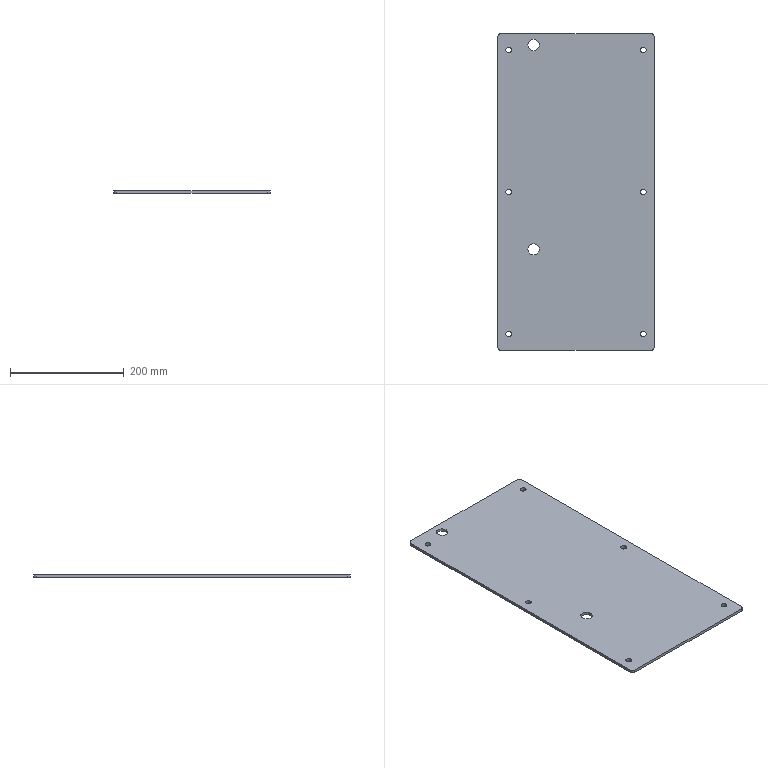Part | SolidWorks | features BaseBody 1 | 1 solid | 26 faces | box 275 x 558 x 5 mm | volume 761645 mm3 | cylinder 20 | plane 6 | commonest cylinder face diameters 10 x16 20 x4
STEP:
#1=CARTESIAN_POINT('',(-64.75,-101.,5.));
#2=VERTEX_POINT('',#1);
#3=CARTESIAN_POINT('',(-84.75,-101.,5.));
#4=VERTEX_POINT('',#3);
#5=CARTESIAN_POINT('',(-74.75,-101.,5.));
#6=DIRECTION('',(0.,0.,-1.));
#7=DIRECTION('',(-1.,0.,0.));
#8=AXIS2_PLACEMENT_3D('',#5,#6,#7);
#9=CIRCLE('',#8,10.);
#10=EDGE_CURVE('',#2,#4,#9,.T.);
#11=ORIENTED_EDGE('',*,*,#10,.F.);
#12=CARTESIAN_POINT('',(-64.75,-101.,0.));
#13=VERTEX_POINT('',#12);
#14=CARTESIAN_POINT('',(-64.75,-101.,10.));
#15=DIRECTION('',(0.,0.,-1.));
#16=VECTOR('',#15,1000.);
#17=LINE('',#14,#16);
#18=EDGE_CURVE('',#2,#13,#17,.T.);
#19=ORIENTED_EDGE('',*,*,#18,.T.);
#20=CARTESIAN_POINT('',(-84.75,-101.,0.));
#21=VERTEX_POINT('',#20);
#22=CARTESIAN_POINT('',(-74.75,-101.,0.));
#23=DIRECTION('',(0.,0.,-1.));
#24=DIRECTION('',(-1.,0.,0.));
#25=AXIS2_PLACEMENT_3D('',#22,#23,#24);
#26=CIRCLE('',#25,10.);
#27=EDGE_CURVE('',#13,#21,#26,.T.);
#28=ORIENTED_EDGE('',*,*,#27,.T.);
#29=CARTESIAN_POINT('',(-84.75,-101.,10.));
#30=DIRECTION('',(0.,0.,-1.));
#31=VECTOR('',#30,1000.);
#32=LINE('',#29,#31);
#33=EDGE_CURVE('',#4,#21,#32,.T.);
#34=ORIENTED_EDGE('',*,*,#33,.F.);
#35=EDGE_LOOP('',(#11,#19,#28,#34));
#36=FACE_OUTER_BOUND('',#35,.T.);
#37=CARTESIAN_POINT('',(-74.75,-101.,10.));
#38=DIRECTION('',(0.,0.,-1.));
#39=DIRECTION('',(-1.,0.,0.));
#40=AXIS2_PLACEMENT_3D('',#37,#38,#39);
#41=CYLINDRICAL_SURFACE('',#40,10.);
#42=ADVANCED_FACE('',(#36),#41,.F.);
#43=CARTESIAN_POINT('',(-64.752,259.,5.));
#44=VERTEX_POINT('',#43);
#45=CARTESIAN_POINT('',(-84.752,259.,5.));
#46=VERTEX_POINT('',#45);
#47=CARTESIAN_POINT('',(-74.752,259.,5.));
#48=DIRECTION('',(0.,0.,-1.));
#49=DIRECTION('',(-1.,0.,0.));
#50=AXIS2_PLACEMENT_3D('',#47,#48,#49);
#51=CIRCLE('',#50,10.);
#52=EDGE_CURVE('',#44,#46,#51,.T.);
#53=ORIENTED_EDGE('',*,*,#52,.F.);
#54=CARTESIAN_POINT('',(-64.752,259.,0.));
#55=VERTEX_POINT('',#54);
#56=CARTESIAN_POINT('',(-64.752,259.,10.));
#57=DIRECTION('',(0.,0.,-1.));
#58=VECTOR('',#57,1000.);
#59=LINE('',#56,#58);
#60=EDGE_CURVE('',#44,#55,#59,.T.);
#61=ORIENTED_EDGE('',*,*,#60,.T.);
#62=CARTESIAN_POINT('',(-84.752,259.,0.));
#63=VERTEX_POINT('',#62);
#64=CARTESIAN_POINT('',(-74.752,259.,0.));
#65=DIRECTION('',(0.,0.,-1.));
#66=DIRECTION('',(-1.,0.,0.));
#67=AXIS2_PLACEMENT_3D('',#64,#65,#66);
#68=CIRCLE('',#67,10.);
#69=EDGE_CURVE('',#55,#63,#68,.T.);
#70=ORIENTED_EDGE('',*,*,#69,.T.);
#71=CARTESIAN_POINT('',(-84.752,259.,10.));
#72=DIRECTION('',(0.,0.,-1.));
#73=VECTOR('',#72,1000.);
#74=LINE('',#71,#73);
#75=EDGE_CURVE('',#46,#63,#74,.T.);
#76=ORIENTED_EDGE('',*,*,#75,.F.);
#77=EDGE_LOOP('',(#53,#61,#70,#76));
#78=FACE_OUTER_BOUND('',#77,.T.);
#79=CARTESIAN_POINT('',(-74.752,259.,10.));
#80=DIRECTION('',(0.,0.,-1.));
#81=DIRECTION('',(-1.,0.,0.));
#82=AXIS2_PLACEMENT_3D('',#79,#80,#81);
#83=CYLINDRICAL_SURFACE('',#82,10.);
#84=ADVANCED_FACE('',(#78),#83,.F.);
#85=CARTESIAN_POINT('',(123.5,250.,5.));
#86=VERTEX_POINT('',#85);
#87=CARTESIAN_POINT('',(113.5,250.,5.));
#88=VERTEX_POINT('',#87);
#89=CARTESIAN_POINT('',(118.5,250.,5.));
#90=DIRECTION('',(0.,0.,-1.));
#91=DIRECTION('',(-1.,0.,0.));
#92=AXIS2_PLACEMENT_3D('',#89,#90,#91);
#93=CIRCLE('',#92,5.);
#94=EDGE_CURVE('',#86,#88,#93,.T.);
#95=ORIENTED_EDGE('',*,*,#94,.F.);
#96=CARTESIAN_POINT('',(123.5,250.,0.));
#97=VERTEX_POINT('',#96);
#98=CARTESIAN_POINT('',(123.5,250.,0.));
#99=DIRECTION('',(0.,0.,-1.));
#100=VECTOR('',#99,1000.);
#101=LINE('',#98,#100);
#102=EDGE_CURVE('',#86,#97,#101,.T.);
#103=ORIENTED_EDGE('',*,*,#102,.T.);
#104=CARTESIAN_POINT('',(113.5,250.,0.));
#105=VERTEX_POINT('',#104);
#106=CARTESIAN_POINT('',(118.5,250.,0.));
#107=DIRECTION('',(0.,0.,-1.));
#108=DIRECTION('',(-1.,0.,0.));
#109=AXIS2_PLACEMENT_3D('',#106,#107,#108);
#110=CIRCLE('',#109,5.);
#111=EDGE_CURVE('',#97,#105,#110,.T.);
#112=ORIENTED_EDGE('',*,*,#111,.T.);
#113=CARTESIAN_POINT('',(113.5,250.,0.));
#114=DIRECTION('',(0.,0.,-1.));
#115=VECTOR('',#114,1000.);
#116=LINE('',#113,#115);
#117=EDGE_CURVE('',#88,#105,#116,.T.);
#118=ORIENTED_EDGE('',*,*,#117,.F.);
#119=EDGE_LOOP('',(#95,#103,#112,#118));
#120=FACE_OUTER_BOUND('',#119,.T.);
#121=CARTESIAN_POINT('',(118.5,250.,0.));
#122=DIRECTION('',(0.,0.,-1.));
#123=DIRECTION('',(-1.,0.,0.));
#124=AXIS2_PLACEMENT_3D('',#121,#122,#123);
#125=CYLINDRICAL_SURFACE('',#124,5.);
#126=ADVANCED_FACE('',(#120),#125,.F.);
#127=CARTESIAN_POINT('',(123.5,0.,5.));
#128=VERTEX_POINT('',#127);
#129=CARTESIAN_POINT('',(113.5,0.,5.));
#130=VERTEX_POINT('',#129);
#131=CARTESIAN_POINT('',(118.5,0.,5.));
#132=DIRECTION('',(0.,0.,-1.));
#133=DIRECTION('',(-1.,0.,0.));
#134=AXIS2_PLACEMENT_3D('',#131,#132,#133);
#135=CIRCLE('',#134,5.);
#136=EDGE_CURVE('',#128,#130,#135,.T.);
#137=ORIENTED_EDGE('',*,*,#136,.F.);
#138=CARTESIAN_POINT('',(123.5,0.,0.));
#139=VERTEX_POINT('',#138);
#140=CARTESIAN_POINT('',(123.5,0.,0.));
#141=DIRECTION('',(0.,0.,-1.));
#142=VECTOR('',#141,1000.);
#143=LINE('',#140,#142);
#144=EDGE_CURVE('',#128,#139,#143,.T.);
#145=ORIENTED_EDGE('',*,*,#144,.T.);
#146=CARTESIAN_POINT('',(113.5,0.,0.));
#147=VERTEX_POINT('',#146);
#148=CARTESIAN_POINT('',(118.5,0.,0.));
#149=DIRECTION('',(0.,0.,-1.));
#150=DIRECTION('',(-1.,0.,0.));
#151=AXIS2_PLACEMENT_3D('',#148,#149,#150);
#152=CIRCLE('',#151,5.);
#153=EDGE_CURVE('',#139,#147,#152,.T.);
#154=ORIENTED_EDGE('',*,*,#153,.T.);
#155=CARTESIAN_POINT('',(113.5,0.,0.));
#156=DIRECTION('',(0.,0.,-1.));
#157=VECTOR('',#156,1000.);
#158=LINE('',#155,#157);
#159=EDGE_CURVE('',#130,#147,#158,.T.);
#160=ORIENTED_EDGE('',*,*,#159,.F.);
#161=EDGE_LOOP('',(#137,#145,#154,#160));
#162=FACE_OUTER_BOUND('',#161,.T.);
#163=CARTESIAN_POINT('',(118.5,0.,0.));
#164=DIRECTION('',(0.,0.,-1.));
#165=DIRECTION('',(-1.,0.,0.));
#166=AXIS2_PLACEMENT_3D('',#163,#164,#165);
#167=CYLINDRICAL_SURFACE('',#166,5.);
#168=ADVANCED_FACE('',(#162),#167,.F.);
#169=CARTESIAN_POINT('',(123.5,-250.,5.));
#170=VERTEX_POINT('',#169);
#171=CARTESIAN_POINT('',(113.5,-250.,5.));
#172=VERTEX_POINT('',#171);
#173=CARTESIAN_POINT('',(118.5,-250.,5.));
#174=DIRECTION('',(0.,0.,-1.));
#175=DIRECTION('',(-1.,0.,0.));
#176=AXIS2_PLACEMENT_3D('',#173,#174,#175);
#177=CIRCLE('',#176,5.);
#178=EDGE_CURVE('',#170,#172,#177,.T.);
#179=ORIENTED_EDGE('',*,*,#178,.F.);
#180=CARTESIAN_POINT('',(123.5,-250.,0.));
#181=VERTEX_POINT('',#180);
#182=CARTESIAN_POINT('',(123.5,-250.,0.));
#183=DIRECTION('',(0.,0.,-1.));
#184=VECTOR('',#183,1000.);
#185=LINE('',#182,#184);
#186=EDGE_CURVE('',#170,#181,#185,.T.);
#187=ORIENTED_EDGE('',*,*,#186,.T.);
#188=CARTESIAN_POINT('',(113.5,-250.,0.));
#189=VERTEX_POINT('',#188);
#190=CARTESIAN_POINT('',(118.5,-250.,0.));
#191=DIRECTION('',(0.,0.,-1.));
#192=DIRECTION('',(-1.,0.,0.));
#193=AXIS2_PLACEMENT_3D('',#190,#191,#192);
#194=CIRCLE('',#193,5.);
#195=EDGE_CURVE('',#181,#189,#194,.T.);
#196=ORIENTED_EDGE('',*,*,#195,.T.);
#197=CARTESIAN_POINT('',(113.5,-250.,0.));
#198=DIRECTION('',(0.,0.,-1.));
#199=VECTOR('',#198,1000.);
#200=LINE('',#197,#199);
#201=EDGE_CURVE('',#172,#189,#200,.T.);
#202=ORIENTED_EDGE('',*,*,#201,.F.);
#203=EDGE_LOOP('',(#179,#187,#196,#202));
#204=FACE_OUTER_BOUND('',#203,.T.);
#205=CARTESIAN_POINT('',(118.5,-250.,0.));
#206=DIRECTION('',(0.,0.,-1.));
#207=DIRECTION('',(-1.,0.,0.));
#208=AXIS2_PLACEMENT_3D('',#205,#206,#207);
#209=CYLINDRICAL_SURFACE('',#208,5.);
#210=ADVANCED_FACE('',(#204),#209,.F.);
#211=CARTESIAN_POINT('',(-113.5,-250.,5.));
#212=VERTEX_POINT('',#211);
#213=CARTESIAN_POINT('',(-123.5,-250.,5.));
#214=VERTEX_POINT('',#213);
#215=CARTESIAN_POINT('',(-118.5,-250.,5.));
#216=DIRECTION('',(0.,0.,-1.));
#217=DIRECTION('',(-1.,0.,0.));
#218=AXIS2_PLACEMENT_3D('',#215,#216,#217);
#219=CIRCLE('',#218,5.);
#220=EDGE_CURVE('',#212,#214,#219,.T.);
#221=ORIENTED_EDGE('',*,*,#220,.F.);
#222=CARTESIAN_POINT('',(-113.5,-250.,0.));
#223=VERTEX_POINT('',#222);
#224=CARTESIAN_POINT('',(-113.5,-250.,0.));
#225=DIRECTION('',(0.,0.,-1.));
#226=VECTOR('',#225,1000.);
#227=LINE('',#224,#226);
#228=EDGE_CURVE('',#212,#223,#227,.T.);
#229=ORIENTED_EDGE('',*,*,#228,.T.);
#230=CARTESIAN_POINT('',(-123.5,-250.,0.));
#231=VERTEX_POINT('',#230);
#232=CARTESIAN_POINT('',(-118.5,-250.,0.));
#233=DIRECTION('',(0.,0.,-1.));
#234=DIRECTION('',(-1.,0.,0.));
#235=AXIS2_PLACEMENT_3D('',#232,#233,#234);
#236=CIRCLE('',#235,5.);
#237=EDGE_CURVE('',#223,#231,#236,.T.);
#238=ORIENTED_EDGE('',*,*,#237,.T.);
#239=CARTESIAN_POINT('',(-123.5,-250.,0.));
#240=DIRECTION('',(0.,0.,-1.));
#241=VECTOR('',#240,1000.);
#242=LINE('',#239,#241);
#243=EDGE_CURVE('',#214,#231,#242,.T.);
#244=ORIENTED_EDGE('',*,*,#243,.F.);
#245=EDGE_LOOP('',(#221,#229,#238,#244));
#246=FACE_OUTER_BOUND('',#245,.T.);
#247=CARTESIAN_POINT('',(-118.5,-250.,0.));
#248=DIRECTION('',(0.,0.,-1.));
#249=DIRECTION('',(-1.,0.,0.));
#250=AXIS2_PLACEMENT_3D('',#247,#248,#249);
#251=CYLINDRICAL_SURFACE('',#250,5.);
#252=ADVANCED_FACE('',(#246),#251,.F.);
#253=CARTESIAN_POINT('',(-113.5,0.,5.));
#254=VERTEX_POINT('',#253);
#255=CARTESIAN_POINT('',(-123.5,0.,5.));
#256=VERTEX_POINT('',#255);
#257=CARTESIAN_POINT('',(-118.5,0.,5.));
#258=DIRECTION('',(0.,0.,-1.));
#259=DIRECTION('',(-1.,0.,0.));
#260=AXIS2_PLACEMENT_3D('',#257,#258,#259);
#261=CIRCLE('',#260,5.);
#262=EDGE_CURVE('',#254,#256,#261,.T.);
#263=ORIENTED_EDGE('',*,*,#262,.F.);
#264=CARTESIAN_POINT('',(-113.5,0.,0.));
#265=VERTEX_POINT('',#264);
#266=CARTESIAN_POINT('',(-113.5,0.,0.));
#267=DIRECTION('',(0.,0.,-1.));
#268=VECTOR('',#267,1000.);
#269=LINE('',#266,#268);
#270=EDGE_CURVE('',#254,#265,#269,.T.);
#271=ORIENTED_EDGE('',*,*,#270,.T.);
#272=CARTESIAN_POINT('',(-123.5,0.,0.));
#273=VERTEX_POINT('',#272);
#274=CARTESIAN_POINT('',(-118.5,0.,0.));
#275=DIRECTION('',(0.,0.,-1.));
#276=DIRECTION('',(-1.,0.,0.));
#277=AXIS2_PLACEMENT_3D('',#274,#275,#276);
#278=CIRCLE('',#277,5.);
#279=EDGE_CURVE('',#265,#273,#278,.T.);
#280=ORIENTED_EDGE('',*,*,#279,.T.);
#281=CARTESIAN_POINT('',(-123.5,0.,0.));
#282=DIRECTION('',(0.,0.,-1.));
#283=VECTOR('',#282,1000.);
#284=LINE('',#281,#283);
#285=EDGE_CURVE('',#256,#273,#284,.T.);
#286=ORIENTED_EDGE('',*,*,#285,.F.);
#287=EDGE_LOOP('',(#263,#271,#280,#286));
#288=FACE_OUTER_BOUND('',#287,.T.);
#289=CARTESIAN_POINT('',(-118.5,0.,0.));
#290=DIRECTION('',(0.,0.,-1.));
#291=DIRECTION('',(-1.,0.,0.));
#292=AXIS2_PLACEMENT_3D('',#289,#290,#291);
#293=CYLINDRICAL_SURFACE('',#292,5.);
#294=ADVANCED_FACE('',(#288),#293,.F.);
#295=CARTESIAN_POINT('',(-113.5,250.,5.));
#296=VERTEX_POINT('',#295);
#297=CARTESIAN_POINT('',(-123.5,250.,5.));
#298=VERTEX_POINT('',#297);
#299=CARTESIAN_POINT('',(-118.5,250.,5.));
#300=DIRECTION('',(0.,0.,-1.));
#301=DIRECTION('',(-1.,0.,0.));
#302=AXIS2_PLACEMENT_3D('',#299,#300,#301);
#303=CIRCLE('',#302,5.);
#304=EDGE_CURVE('',#296,#298,#303,.T.);
#305=ORIENTED_EDGE('',*,*,#304,.F.);
#306=CARTESIAN_POINT('',(-113.5,250.,0.));
#307=VERTEX_POINT('',#306);
#308=CARTESIAN_POINT('',(-113.5,250.,0.));
#309=DIRECTION('',(0.,0.,-1.));
#310=VECTOR('',#309,1000.);
#311=LINE('',#308,#310);
#312=EDGE_CURVE('',#296,#307,#311,.T.);
#313=ORIENTED_EDGE('',*,*,#312,.T.);
#314=CARTESIAN_POINT('',(-123.5,250.,0.));
#315=VERTEX_POINT('',#314);
#316=CARTESIAN_POINT('',(-118.5,250.,0.));
#317=DIRECTION('',(0.,0.,-1.));
#318=DIRECTION('',(-1.,0.,0.));
#319=AXIS2_PLACEMENT_3D('',#316,#317,#318);
#320=CIRCLE('',#319,5.);
#321=EDGE_CURVE('',#307,#315,#320,.T.);
#322=ORIENTED_EDGE('',*,*,#321,.T.);
#323=CARTESIAN_POINT('',(-123.5,250.,0.));
#324=DIRECTION('',(0.,0.,-1.));
#325=VECTOR('',#324,1000.);
#326=LINE('',#323,#325);
#327=EDGE_CURVE('',#298,#315,#326,.T.);
#328=ORIENTED_EDGE('',*,*,#327,.F.);
#329=EDGE_LOOP('',(#305,#313,#322,#328));
#330=FACE_OUTER_BOUND('',#329,.T.);
#331=CARTESIAN_POINT('',(-118.5,250.,0.));
#332=DIRECTION('',(0.,0.,-1.));
#333=DIRECTION('',(-1.,0.,0.));
#334=AXIS2_PLACEMENT_3D('',#331,#332,#333);
#335=CYLINDRICAL_SURFACE('',#334,5.);
#336=ADVANCED_FACE('',(#330),#335,.F.);
#337=CARTESIAN_POINT('',(-137.5,274.,0.));
#338=VERTEX_POINT('',#337);
#339=CARTESIAN_POINT('',(-137.5,-274.,0.));
#340=VERTEX_POINT('',#339);
#341=CARTESIAN_POINT('',(-137.5,279.,0.));
#342=DIRECTION('',(0.,-1.,0.));
#343=VECTOR('',#342,1000.);
#344=LINE('',#341,#343);
#345=EDGE_CURVE('',#338,#340,#344,.T.);
#346=ORIENTED_EDGE('',*,*,#345,.T.);
#347=CARTESIAN_POINT('',(-137.5,-274.,5.));
#348=VERTEX_POINT('',#347);
#349=CARTESIAN_POINT('',(-137.5,-274.,5.));
#350=DIRECTION('',(0.,0.,1.));
#351=VECTOR('',#350,1000.);
#352=LINE('',#349,#351);
#353=EDGE_CURVE('',#340,#348,#352,.T.);
#354=ORIENTED_EDGE('',*,*,#353,.T.);
#355=CARTESIAN_POINT('',(-137.5,274.,5.));
#356=VERTEX_POINT('',#355);
#357=CARTESIAN_POINT('',(-137.5,279.,5.));
#358=DIRECTION('',(0.,-1.,0.));
#359=VECTOR('',#358,1000.);
#360=LINE('',#357,#359);
#361=EDGE_CURVE('',#356,#348,#360,.T.);
#362=ORIENTED_EDGE('',*,*,#361,.F.);
#363=CARTESIAN_POINT('',(-137.5,274.,5.));
#364=DIRECTION('',(0.,0.,-1.));
#365=VECTOR('',#364,1000.);
#366=LINE('',#363,#365);
#367=EDGE_CURVE('',#356,#338,#366,.T.);
#368=ORIENTED_EDGE('',*,*,#367,.T.);
#369=EDGE_LOOP('',(#346,#354,#362,#368));
#370=FACE_OUTER_BOUND('',#369,.T.);
#371=CARTESIAN_POINT('',(-137.5,279.,5.));
#372=DIRECTION('',(1.,0.,0.));
#373=DIRECTION('',(0.,1.,0.));
#374=AXIS2_PLACEMENT_3D('',#371,#372,#373);
#375=PLANE('',#374);
#376=ADVANCED_FACE('',(#370),#375,.F.);
#377=CARTESIAN_POINT('',(-132.5,-279.,0.));
#378=VERTEX_POINT('',#377);
#379=CARTESIAN_POINT('',(132.5,-279.,0.));
#380=VERTEX_POINT('',#379);
#381=CARTESIAN_POINT('',(137.5,-279.,0.));
#382=DIRECTION('',(1.,0.,0.));
#383=VECTOR('',#382,1000.);
#384=LINE('',#381,#383);
#385=EDGE_CURVE('',#378,#380,#384,.T.);
#386=ORIENTED_EDGE('',*,*,#385,.T.);
#387=CARTESIAN_POINT('',(132.5,-279.,5.));
#388=VERTEX_POINT('',#387);
#389=CARTESIAN_POINT('',(132.5,-279.,5.));
#390=DIRECTION('',(0.,0.,1.));
#391=VECTOR('',#390,1000.);
#392=LINE('',#389,#391);
#393=EDGE_CURVE('',#380,#388,#392,.T.);
#394=ORIENTED_EDGE('',*,*,#393,.T.);
#395=CARTESIAN_POINT('',(-132.5,-279.,5.));
#396=VERTEX_POINT('',#395);
#397=CARTESIAN_POINT('',(137.5,-279.,5.));
#398=DIRECTION('',(1.,0.,0.));
#399=VECTOR('',#398,1000.);
#400=LINE('',#397,#399);
#401=EDGE_CURVE('',#396,#388,#400,.T.);
#402=ORIENTED_EDGE('',*,*,#401,.F.);
#403=CARTESIAN_POINT('',(-132.5,-279.,5.));
#404=DIRECTION('',(0.,0.,-1.));
#405=VECTOR('',#404,1000.);
#406=LINE('',#403,#405);
#407=EDGE_CURVE('',#396,#378,#406,.T.);
#408=ORIENTED_EDGE('',*,*,#407,.T.);
#409=EDGE_LOOP('',(#386,#394,#402,#408));
#410=FACE_OUTER_BOUND('',#409,.T.);
#411=CARTESIAN_POINT('',(137.5,-279.,5.));
#412=DIRECTION('',(0.,1.,0.));
#413=DIRECTION('',(0.,0.,1.));
#414=AXIS2_PLACEMENT_3D('',#411,#412,#413);
#415=PLANE('',#414);
#416=ADVANCED_FACE('',(#410),#415,.F.);
#417=CARTESIAN_POINT('',(137.5,-274.,5.));
#418=VERTEX_POINT('',#417);
#419=CARTESIAN_POINT('',(137.5,274.,5.));
#420=VERTEX_POINT('',#419);
#421=CARTESIAN_POINT('',(137.5,279.,5.));
#422=DIRECTION('',(0.,1.,0.));
#423=VECTOR('',#422,1000.);
#424=LINE('',#421,#423);
#425=EDGE_CURVE('',#418,#420,#424,.T.);
#426=ORIENTED_EDGE('',*,*,#425,.F.);
#427=CARTESIAN_POINT('',(137.5,-274.,0.));
#428=VERTEX_POINT('',#427);
#429=CARTESIAN_POINT('',(137.5,-274.,5.));
#430=DIRECTION('',(0.,0.,-1.));
#431=VECTOR('',#430,1000.);
#432=LINE('',#429,#431);
#433=EDGE_CURVE('',#418,#428,#432,.T.);
#434=ORIENTED_EDGE('',*,*,#433,.T.);
#435=CARTESIAN_POINT('',(137.5,274.,0.));
#436=VERTEX_POINT('',#435);
#437=CARTESIAN_POINT('',(137.5,279.,0.));
#438=DIRECTION('',(0.,1.,0.));
#439=VECTOR('',#438,1000.);
#440=LINE('',#437,#439);
#441=EDGE_CURVE('',#428,#436,#440,.T.);
#442=ORIENTED_EDGE('',*,*,#441,.T.);
#443=CARTESIAN_POINT('',(137.5,274.,5.));
#444=DIRECTION('',(0.,0.,1.));
#445=VECTOR('',#444,1000.);
#446=LINE('',#443,#445);
#447=EDGE_CURVE('',#436,#420,#446,.T.);
#448=ORIENTED_EDGE('',*,*,#447,.T.);
#449=EDGE_LOOP('',(#426,#434,#442,#448));
#450=FACE_OUTER_BOUND('',#449,.T.);
#451=CARTESIAN_POINT('',(137.5,279.,5.));
#452=DIRECTION('',(-1.,0.,0.));
#453=DIRECTION('',(0.,-1.,0.));
#454=AXIS2_PLACEMENT_3D('',#451,#452,#453);
#455=PLANE('',#454);
#456=ADVANCED_FACE('',(#450),#455,.F.);
#457=CARTESIAN_POINT('',(132.5,279.,5.));
#458=VERTEX_POINT('',#457);
#459=CARTESIAN_POINT('',(-132.5,279.,5.));
#460=VERTEX_POINT('',#459);
#461=CARTESIAN_POINT('',(137.5,279.,5.));
#462=DIRECTION('',(-1.,0.,0.));
#463=VECTOR('',#462,1000.);
#464=LINE('',#461,#463);
#465=EDGE_CURVE('',#458,#460,#464,.T.);
#466=ORIENTED_EDGE('',*,*,#465,.F.);
#467=CARTESIAN_POINT('',(132.5,279.,0.));
#468=VERTEX_POINT('',#467);
#469=CARTESIAN_POINT('',(132.5,279.,5.));
#470=DIRECTION('',(0.,0.,-1.));
#471=VECTOR('',#470,1000.);
#472=LINE('',#469,#471);
#473=EDGE_CURVE('',#458,#468,#472,.T.);
#474=ORIENTED_EDGE('',*,*,#473,.T.);
#475=CARTESIAN_POINT('',(-132.5,279.,0.));
#476=VERTEX_POINT('',#475);
#477=CARTESIAN_POINT('',(137.5,279.,0.));
#478=DIRECTION('',(-1.,0.,0.));
#479=VECTOR('',#478,1000.);
#480=LINE('',#477,#479);
#481=EDGE_CURVE('',#468,#476,#480,.T.);
#482=ORIENTED_EDGE('',*,*,#481,.T.);
#483=CARTESIAN_POINT('',(-132.5,279.,5.));
#484=DIRECTION('',(0.,0.,1.));
#485=VECTOR('',#484,1000.);
#486=LINE('',#483,#485);
#487=EDGE_CURVE('',#476,#460,#486,.T.);
#488=ORIENTED_EDGE('',*,*,#487,.T.);
#489=EDGE_LOOP('',(#466,#474,#482,#488));
#490=FACE_OUTER_BOUND('',#489,.T.);
#491=CARTESIAN_POINT('',(137.5,279.,5.));
#492=DIRECTION('',(0.,-1.,0.));
#493=DIRECTION('',(1.,0.,0.));
#494=AXIS2_PLACEMENT_3D('',#491,#492,#493);
#495=PLANE('',#494);
#496=ADVANCED_FACE('',(#490),#495,.F.);
#497=CARTESIAN_POINT('',(-74.75,-101.,5.));
#498=DIRECTION('',(0.,0.,-1.));
#499=DIRECTION('',(-1.,0.,0.));
#500=AXIS2_PLACEMENT_3D('',#497,#498,#499);
#501=CIRCLE('',#500,10.);
#502=EDGE_CURVE('',#4,#2,#501,.T.);
#503=ORIENTED_EDGE('',*,*,#502,.T.);
#504=ORIENTED_EDGE('',*,*,#10,.T.);
#505=EDGE_LOOP('',(#503,#504));
#506=FACE_BOUND('',#505,.T.);
#507=CARTESIAN_POINT('',(-74.752,259.,5.));
#508=DIRECTION('',(0.,0.,-1.));
#509=DIRECTION('',(-1.,0.,0.));
#510=AXIS2_PLACEMENT_3D('',#507,#508,#509);
#511=CIRCLE('',#510,10.);
#512=EDGE_CURVE('',#46,#44,#511,.T.);
#513=ORIENTED_EDGE('',*,*,#512,.T.);
#514=ORIENTED_EDGE('',*,*,#52,.T.);
#515=EDGE_LOOP('',(#513,#514));
#516=FACE_BOUND('',#515,.T.);
#517=CARTESIAN_POINT('',(118.5,250.,5.));
#518=DIRECTION('',(0.,0.,-1.));
#519=DIRECTION('',(-1.,0.,0.));
#520=AXIS2_PLACEMENT_3D('',#517,#518,#519);
#521=CIRCLE('',#520,5.);
#522=EDGE_CURVE('',#88,#86,#521,.T.);
#523=ORIENTED_EDGE('',*,*,#522,.T.);
#524=ORIENTED_EDGE('',*,*,#94,.T.);
#525=EDGE_LOOP('',(#523,#524));
#526=FACE_BOUND('',#525,.T.);
#527=CARTESIAN_POINT('',(118.5,0.,5.));
#528=DIRECTION('',(0.,0.,-1.));
#529=DIRECTION('',(-1.,0.,0.));
#530=AXIS2_PLACEMENT_3D('',#527,#528,#529);
#531=CIRCLE('',#530,5.);
#532=EDGE_CURVE('',#130,#128,#531,.T.);
#533=ORIENTED_EDGE('',*,*,#532,.T.);
#534=ORIENTED_EDGE('',*,*,#136,.T.);
#535=EDGE_LOOP('',(#533,#534));
#536=FACE_BOUND('',#535,.T.);
#537=CARTESIAN_POINT('',(118.5,-250.,5.));
#538=DIRECTION('',(0.,0.,-1.));
#539=DIRECTION('',(-1.,0.,0.));
#540=AXIS2_PLACEMENT_3D('',#537,#538,#539);
#541=CIRCLE('',#540,5.);
#542=EDGE_CURVE('',#172,#170,#541,.T.);
#543=ORIENTED_EDGE('',*,*,#542,.T.);
#544=ORIENTED_EDGE('',*,*,#178,.T.);
#545=EDGE_LOOP('',(#543,#544));
#546=FACE_BOUND('',#545,.T.);
#547=CARTESIAN_POINT('',(-118.5,-250.,5.));
#548=DIRECTION('',(0.,0.,-1.));
#549=DIRECTION('',(-1.,0.,0.));
#550=AXIS2_PLACEMENT_3D('',#547,#548,#549);
#551=CIRCLE('',#550,5.);
#552=EDGE_CURVE('',#214,#212,#551,.T.);
#553=ORIENTED_EDGE('',*,*,#552,.T.);
#554=ORIENTED_EDGE('',*,*,#220,.T.);
#555=EDGE_LOOP('',(#553,#554));
#556=FACE_BOUND('',#555,.T.);
#557=CARTESIAN_POINT('',(-118.5,0.,5.));
#558=DIRECTION('',(0.,0.,-1.));
#559=DIRECTION('',(-1.,0.,0.));
#560=AXIS2_PLACEMENT_3D('',#557,#558,#559);
#561=CIRCLE('',#560,5.);
#562=EDGE_CURVE('',#256,#254,#561,.T.);
#563=ORIENTED_EDGE('',*,*,#562,.T.);
#564=ORIENTED_EDGE('',*,*,#262,.T.);
#565=EDGE_LOOP('',(#563,#564));
#566=FACE_BOUND('',#565,.T.);
#567=CARTESIAN_POINT('',(-118.5,250.,5.));
#568=DIRECTION('',(0.,0.,-1.));
#569=DIRECTION('',(-1.,0.,0.));
#570=AXIS2_PLACEMENT_3D('',#567,#568,#569);
#571=CIRCLE('',#570,5.);
#572=EDGE_CURVE('',#298,#296,#571,.T.);
#573=ORIENTED_EDGE('',*,*,#572,.T.);
#574=ORIENTED_EDGE('',*,*,#304,.T.);
#575=EDGE_LOOP('',(#573,#574));
#576=FACE_BOUND('',#575,.T.);
#577=ORIENTED_EDGE('',*,*,#401,.T.);
#578=CARTESIAN_POINT('',(132.5,-274.,5.));
#579=DIRECTION('',(0.,0.,1.));
#580=DIRECTION('',(-1.,0.,0.));
#581=AXIS2_PLACEMENT_3D('',#578,#579,#580);
#582=CIRCLE('',#581,5.);
#583=EDGE_CURVE('',#388,#418,#582,.T.);
#584=ORIENTED_EDGE('',*,*,#583,.T.);
#585=ORIENTED_EDGE('',*,*,#425,.T.);
#586=CARTESIAN_POINT('',(132.5,274.,5.));
#587=DIRECTION('',(0.,0.,1.));
#588=DIRECTION('',(-1.,0.,0.));
#589=AXIS2_PLACEMENT_3D('',#586,#587,#588);
#590=CIRCLE('',#589,5.);
#591=EDGE_CURVE('',#420,#458,#590,.T.);
#592=ORIENTED_EDGE('',*,*,#591,.T.);
#593=ORIENTED_EDGE('',*,*,#465,.T.);
#594=CARTESIAN_POINT('',(-132.5,274.,5.));
#595=DIRECTION('',(0.,0.,1.));
#596=DIRECTION('',(-1.,0.,0.));
#597=AXIS2_PLACEMENT_3D('',#594,#595,#596);
#598=CIRCLE('',#597,5.);
#599=EDGE_CURVE('',#460,#356,#598,.T.);
#600=ORIENTED_EDGE('',*,*,#599,.T.);
#601=ORIENTED_EDGE('',*,*,#361,.T.);
#602=CARTESIAN_POINT('',(-132.5,-274.,5.));
#603=DIRECTION('',(0.,0.,1.));
#604=DIRECTION('',(-1.,0.,0.));
#605=AXIS2_PLACEMENT_3D('',#602,#603,#604);
#606=CIRCLE('',#605,5.);
#607=EDGE_CURVE('',#348,#396,#606,.T.);
#608=ORIENTED_EDGE('',*,*,#607,.T.);
#609=EDGE_LOOP('',(#577,#584,#585,#592,#593,#600,#601,#608));
#610=FACE_OUTER_BOUND('',#609,.T.);
#611=CARTESIAN_POINT('',(0.,0.,5.));
#612=DIRECTION('',(0.,0.,-1.));
#613=DIRECTION('',(-1.,0.,0.));
#614=AXIS2_PLACEMENT_3D('',#611,#612,#613);
#615=PLANE('',#614);
#616=ADVANCED_FACE('',(#506,#516,#526,#536,#546,#556,#566,#576,#610),#615,.F.);
#617=CARTESIAN_POINT('',(-74.75,-101.,0.));
#618=DIRECTION('',(0.,0.,-1.));
#619=DIRECTION('',(-1.,0.,0.));
#620=AXIS2_PLACEMENT_3D('',#617,#618,#619);
#621=CIRCLE('',#620,10.);
#622=EDGE_CURVE('',#21,#13,#621,.T.);
#623=ORIENTED_EDGE('',*,*,#622,.F.);
#624=ORIENTED_EDGE('',*,*,#27,.F.);
#625=EDGE_LOOP('',(#623,#624));
#626=FACE_BOUND('',#625,.T.);
#627=CARTESIAN_POINT('',(-74.752,259.,0.));
#628=DIRECTION('',(0.,0.,-1.));
#629=DIRECTION('',(-1.,0.,0.));
#630=AXIS2_PLACEMENT_3D('',#627,#628,#629);
#631=CIRCLE('',#630,10.);
#632=EDGE_CURVE('',#63,#55,#631,.T.);
#633=ORIENTED_EDGE('',*,*,#632,.F.);
#634=ORIENTED_EDGE('',*,*,#69,.F.);
#635=EDGE_LOOP('',(#633,#634));
#636=FACE_BOUND('',#635,.T.);
#637=CARTESIAN_POINT('',(118.5,250.,0.));
#638=DIRECTION('',(0.,0.,-1.));
#639=DIRECTION('',(-1.,0.,0.));
#640=AXIS2_PLACEMENT_3D('',#637,#638,#639);
#641=CIRCLE('',#640,5.);
#642=EDGE_CURVE('',#105,#97,#641,.T.);
#643=ORIENTED_EDGE('',*,*,#642,.F.);
#644=ORIENTED_EDGE('',*,*,#111,.F.);
#645=EDGE_LOOP('',(#643,#644));
#646=FACE_BOUND('',#645,.T.);
#647=CARTESIAN_POINT('',(118.5,0.,0.));
#648=DIRECTION('',(0.,0.,-1.));
#649=DIRECTION('',(-1.,0.,0.));
#650=AXIS2_PLACEMENT_3D('',#647,#648,#649);
#651=CIRCLE('',#650,5.);
#652=EDGE_CURVE('',#147,#139,#651,.T.);
#653=ORIENTED_EDGE('',*,*,#652,.F.);
#654=ORIENTED_EDGE('',*,*,#153,.F.);
#655=EDGE_LOOP('',(#653,#654));
#656=FACE_BOUND('',#655,.T.);
#657=CARTESIAN_POINT('',(118.5,-250.,0.));
#658=DIRECTION('',(0.,0.,-1.));
#659=DIRECTION('',(-1.,0.,0.));
#660=AXIS2_PLACEMENT_3D('',#657,#658,#659);
#661=CIRCLE('',#660,5.);
#662=EDGE_CURVE('',#189,#181,#661,.T.);
#663=ORIENTED_EDGE('',*,*,#662,.F.);
#664=ORIENTED_EDGE('',*,*,#195,.F.);
#665=EDGE_LOOP('',(#663,#664));
#666=FACE_BOUND('',#665,.T.);
#667=CARTESIAN_POINT('',(-118.5,-250.,0.));
#668=DIRECTION('',(0.,0.,-1.));
#669=DIRECTION('',(-1.,0.,0.));
#670=AXIS2_PLACEMENT_3D('',#667,#668,#669);
#671=CIRCLE('',#670,5.);
#672=EDGE_CURVE('',#231,#223,#671,.T.);
#673=ORIENTED_EDGE('',*,*,#672,.F.);
#674=ORIENTED_EDGE('',*,*,#237,.F.);
#675=EDGE_LOOP('',(#673,#674));
#676=FACE_BOUND('',#675,.T.);
#677=CARTESIAN_POINT('',(-118.5,0.,0.));
#678=DIRECTION('',(0.,0.,-1.));
#679=DIRECTION('',(-1.,0.,0.));
#680=AXIS2_PLACEMENT_3D('',#677,#678,#679);
#681=CIRCLE('',#680,5.);
#682=EDGE_CURVE('',#273,#265,#681,.T.);
#683=ORIENTED_EDGE('',*,*,#682,.F.);
#684=ORIENTED_EDGE('',*,*,#279,.F.);
#685=EDGE_LOOP('',(#683,#684));
#686=FACE_BOUND('',#685,.T.);
#687=CARTESIAN_POINT('',(-118.5,250.,0.));
#688=DIRECTION('',(0.,0.,-1.));
#689=DIRECTION('',(-1.,0.,0.));
#690=AXIS2_PLACEMENT_3D('',#687,#688,#689);
#691=CIRCLE('',#690,5.);
#692=EDGE_CURVE('',#315,#307,#691,.T.);
#693=ORIENTED_EDGE('',*,*,#692,.F.);
#694=ORIENTED_EDGE('',*,*,#321,.F.);
#695=EDGE_LOOP('',(#693,#694));
#696=FACE_BOUND('',#695,.T.);
#697=ORIENTED_EDGE('',*,*,#441,.F.);
#698=CARTESIAN_POINT('',(132.5,-274.,0.));
#699=DIRECTION('',(0.,0.,-1.));
#700=DIRECTION('',(-1.,0.,0.));
#701=AXIS2_PLACEMENT_3D('',#698,#699,#700);
#702=CIRCLE('',#701,5.);
#703=EDGE_CURVE('',#428,#380,#702,.T.);
#704=ORIENTED_EDGE('',*,*,#703,.T.);
#705=ORIENTED_EDGE('',*,*,#385,.F.);
#706=CARTESIAN_POINT('',(-132.5,-274.,0.));
#707=DIRECTION('',(0.,0.,-1.));
#708=DIRECTION('',(-1.,0.,0.));
#709=AXIS2_PLACEMENT_3D('',#706,#707,#708);
#710=CIRCLE('',#709,5.);
#711=EDGE_CURVE('',#378,#340,#710,.T.);
#712=ORIENTED_EDGE('',*,*,#711,.T.);
#713=ORIENTED_EDGE('',*,*,#345,.F.);
#714=CARTESIAN_POINT('',(-132.5,274.,0.));
#715=DIRECTION('',(0.,0.,-1.));
#716=DIRECTION('',(-1.,0.,0.));
#717=AXIS2_PLACEMENT_3D('',#714,#715,#716);
#718=CIRCLE('',#717,5.);
#719=EDGE_CURVE('',#338,#476,#718,.T.);
#720=ORIENTED_EDGE('',*,*,#719,.T.);
#721=ORIENTED_EDGE('',*,*,#481,.F.);
#722=CARTESIAN_POINT('',(132.5,274.,0.));
#723=DIRECTION('',(0.,0.,-1.));
#724=DIRECTION('',(-1.,0.,0.));
#725=AXIS2_PLACEMENT_3D('',#722,#723,#724);
#726=CIRCLE('',#725,5.);
#727=EDGE_CURVE('',#468,#436,#726,.T.);
#728=ORIENTED_EDGE('',*,*,#727,.T.);
#729=EDGE_LOOP('',(#697,#704,#705,#712,#713,#720,#721,#728));
#730=FACE_OUTER_BOUND('',#729,.T.);
#731=CARTESIAN_POINT('',(0.,0.,0.));
#732=DIRECTION('',(0.,0.,-1.));
#733=DIRECTION('',(-1.,0.,0.));
#734=AXIS2_PLACEMENT_3D('',#731,#732,#733);
#735=PLANE('',#734);
#736=ADVANCED_FACE('',(#626,#636,#646,#656,#666,#676,#686,#696,#730),#735,.T.);
#737=ORIENTED_EDGE('',*,*,#583,.F.);
#738=ORIENTED_EDGE('',*,*,#393,.F.);
#739=ORIENTED_EDGE('',*,*,#703,.F.);
#740=ORIENTED_EDGE('',*,*,#433,.F.);
#741=EDGE_LOOP('',(#737,#738,#739,#740));
#742=FACE_OUTER_BOUND('',#741,.T.);
#743=CARTESIAN_POINT('',(132.5,-274.,5.));
#744=DIRECTION('',(0.,0.,-1.));
#745=DIRECTION('',(-1.,0.,0.));
#746=AXIS2_PLACEMENT_3D('',#743,#744,#745);
#747=CYLINDRICAL_SURFACE('',#746,5.);
#748=ADVANCED_FACE('',(#742),#747,.T.);
#749=ORIENTED_EDGE('',*,*,#607,.F.);
#750=ORIENTED_EDGE('',*,*,#353,.F.);
#751=ORIENTED_EDGE('',*,*,#711,.F.);
#752=ORIENTED_EDGE('',*,*,#407,.F.);
#753=EDGE_LOOP('',(#749,#750,#751,#752));
#754=FACE_OUTER_BOUND('',#753,.T.);
#755=CARTESIAN_POINT('',(-132.5,-274.,5.));
#756=DIRECTION('',(0.,0.,-1.));
#757=DIRECTION('',(-1.,0.,0.));
#758=AXIS2_PLACEMENT_3D('',#755,#756,#757);
#759=CYLINDRICAL_SURFACE('',#758,5.);
#760=ADVANCED_FACE('',(#754),#759,.T.);
#761=ORIENTED_EDGE('',*,*,#591,.F.);
#762=ORIENTED_EDGE('',*,*,#447,.F.);
#763=ORIENTED_EDGE('',*,*,#727,.F.);
#764=ORIENTED_EDGE('',*,*,#473,.F.);
#765=EDGE_LOOP('',(#761,#762,#763,#764));
#766=FACE_OUTER_BOUND('',#765,.T.);
#767=CARTESIAN_POINT('',(132.5,274.,5.));
#768=DIRECTION('',(0.,0.,-1.));
#769=DIRECTION('',(-1.,0.,0.));
#770=AXIS2_PLACEMENT_3D('',#767,#768,#769);
#771=CYLINDRICAL_SURFACE('',#770,5.);
#772=ADVANCED_FACE('',(#766),#771,.T.);
#773=ORIENTED_EDGE('',*,*,#599,.F.);
#774=ORIENTED_EDGE('',*,*,#487,.F.);
#775=ORIENTED_EDGE('',*,*,#719,.F.);
#776=ORIENTED_EDGE('',*,*,#367,.F.);
#777=EDGE_LOOP('',(#773,#774,#775,#776));
#778=FACE_OUTER_BOUND('',#777,.T.);
#779=CARTESIAN_POINT('',(-132.5,274.,5.));
#780=DIRECTION('',(0.,0.,-1.));
#781=DIRECTION('',(-1.,0.,0.));
#782=AXIS2_PLACEMENT_3D('',#779,#780,#781);
#783=CYLINDRICAL_SURFACE('',#782,5.);
#784=ADVANCED_FACE('',(#778),#783,.T.);
#785=ORIENTED_EDGE('',*,*,#312,.F.);
#786=ORIENTED_EDGE('',*,*,#572,.F.);
#787=ORIENTED_EDGE('',*,*,#327,.T.);
#788=ORIENTED_EDGE('',*,*,#692,.T.);
#789=EDGE_LOOP('',(#785,#786,#787,#788));
#790=FACE_OUTER_BOUND('',#789,.T.);
#791=CARTESIAN_POINT('',(-118.5,250.,0.));
#792=DIRECTION('',(0.,0.,-1.));
#793=DIRECTION('',(-1.,0.,0.));
#794=AXIS2_PLACEMENT_3D('',#791,#792,#793);
#795=CYLINDRICAL_SURFACE('',#794,5.);
#796=ADVANCED_FACE('',(#790),#795,.F.);
#797=ORIENTED_EDGE('',*,*,#270,.F.);
#798=ORIENTED_EDGE('',*,*,#562,.F.);
#799=ORIENTED_EDGE('',*,*,#285,.T.);
#800=ORIENTED_EDGE('',*,*,#682,.T.);
#801=EDGE_LOOP('',(#797,#798,#799,#800));
#802=FACE_OUTER_BOUND('',#801,.T.);
#803=CARTESIAN_POINT('',(-118.5,0.,0.));
#804=DIRECTION('',(0.,0.,-1.));
#805=DIRECTION('',(-1.,0.,0.));
#806=AXIS2_PLACEMENT_3D('',#803,#804,#805);
#807=CYLINDRICAL_SURFACE('',#806,5.);
#808=ADVANCED_FACE('',(#802),#807,.F.);
#809=ORIENTED_EDGE('',*,*,#228,.F.);
#810=ORIENTED_EDGE('',*,*,#552,.F.);
#811=ORIENTED_EDGE('',*,*,#243,.T.);
#812=ORIENTED_EDGE('',*,*,#672,.T.);
#813=EDGE_LOOP('',(#809,#810,#811,#812));
#814=FACE_OUTER_BOUND('',#813,.T.);
#815=CARTESIAN_POINT('',(-118.5,-250.,0.));
#816=DIRECTION('',(0.,0.,-1.));
#817=DIRECTION('',(-1.,0.,0.));
#818=AXIS2_PLACEMENT_3D('',#815,#816,#817);
#819=CYLINDRICAL_SURFACE('',#818,5.);
#820=ADVANCED_FACE('',(#814),#819,.F.);
#821=ORIENTED_EDGE('',*,*,#186,.F.);
#822=ORIENTED_EDGE('',*,*,#542,.F.);
#823=ORIENTED_EDGE('',*,*,#201,.T.);
#824=ORIENTED_EDGE('',*,*,#662,.T.);
#825=EDGE_LOOP('',(#821,#822,#823,#824));
#826=FACE_OUTER_BOUND('',#825,.T.);
#827=CARTESIAN_POINT('',(118.5,-250.,0.));
#828=DIRECTION('',(0.,0.,-1.));
#829=DIRECTION('',(-1.,0.,0.));
#830=AXIS2_PLACEMENT_3D('',#827,#828,#829);
#831=CYLINDRICAL_SURFACE('',#830,5.);
#832=ADVANCED_FACE('',(#826),#831,.F.);
#833=ORIENTED_EDGE('',*,*,#144,.F.);
#834=ORIENTED_EDGE('',*,*,#532,.F.);
#835=ORIENTED_EDGE('',*,*,#159,.T.);
#836=ORIENTED_EDGE('',*,*,#652,.T.);
#837=EDGE_LOOP('',(#833,#834,#835,#836));
#838=FACE_OUTER_BOUND('',#837,.T.);
#839=CARTESIAN_POINT('',(118.5,0.,0.));
#840=DIRECTION('',(0.,0.,-1.));
#841=DIRECTION('',(-1.,0.,0.));
#842=AXIS2_PLACEMENT_3D('',#839,#840,#841);
#843=CYLINDRICAL_SURFACE('',#842,5.);
#844=ADVANCED_FACE('',(#838),#843,.F.);
#845=ORIENTED_EDGE('',*,*,#102,.F.);
#846=ORIENTED_EDGE('',*,*,#522,.F.);
#847=ORIENTED_EDGE('',*,*,#117,.T.);
#848=ORIENTED_EDGE('',*,*,#642,.T.);
#849=EDGE_LOOP('',(#845,#846,#847,#848));
#850=FACE_OUTER_BOUND('',#849,.T.);
#851=CARTESIAN_POINT('',(118.5,250.,0.));
#852=DIRECTION('',(0.,0.,-1.));
#853=DIRECTION('',(-1.,0.,0.));
#854=AXIS2_PLACEMENT_3D('',#851,#852,#853);
#855=CYLINDRICAL_SURFACE('',#854,5.);
#856=ADVANCED_FACE('',(#850),#855,.F.);
#857=ORIENTED_EDGE('',*,*,#60,.F.);
#858=ORIENTED_EDGE('',*,*,#512,.F.);
#859=ORIENTED_EDGE('',*,*,#75,.T.);
#860=ORIENTED_EDGE('',*,*,#632,.T.);
#861=EDGE_LOOP('',(#857,#858,#859,#860));
#862=FACE_OUTER_BOUND('',#861,.T.);
#863=CARTESIAN_POINT('',(-74.752,259.,10.));
#864=DIRECTION('',(0.,0.,-1.));
#865=DIRECTION('',(-1.,0.,0.));
#866=AXIS2_PLACEMENT_3D('',#863,#864,#865);
#867=CYLINDRICAL_SURFACE('',#866,10.);
#868=ADVANCED_FACE('',(#862),#867,.F.);
#869=ORIENTED_EDGE('',*,*,#18,.F.);
#870=ORIENTED_EDGE('',*,*,#502,.F.);
#871=ORIENTED_EDGE('',*,*,#33,.T.);
#872=ORIENTED_EDGE('',*,*,#622,.T.);
#873=EDGE_LOOP('',(#869,#870,#871,#872));
#874=FACE_OUTER_BOUND('',#873,.T.);
#875=CARTESIAN_POINT('',(-74.75,-101.,10.));
#876=DIRECTION('',(0.,0.,-1.));
#877=DIRECTION('',(-1.,0.,0.));
#878=AXIS2_PLACEMENT_3D('',#875,#876,#877);
#879=CYLINDRICAL_SURFACE('',#878,10.);
#880=ADVANCED_FACE('',(#874),#879,.F.);
#881=CLOSED_SHELL('',(#42,#84,#126,#168,#210,#252,#294,#336,#376,#416,#456,#496,#616,#736,#748,#760,#772,#784,#796,#808,#820,#832,#844,#856,#868,#880));
#882=MANIFOLD_SOLID_BREP('',#881);
#883=CARTESIAN_POINT('',(0.,0.,0.));
#884=DIRECTION('',(0.,0.,1.));
#885=DIRECTION('',(1.,0.,0.));
#886=AXIS2_PLACEMENT_3D('',#883,#884,#885);
#887=(LENGTH_UNIT()NAMED_UNIT(*)SI_UNIT(.MILLI.,.METRE.));
#888=UNCERTAINTY_MEASURE_WITH_UNIT(LENGTH_MEASURE(0.00001),#887,'','');
#889=(NAMED_UNIT(*)PLANE_ANGLE_UNIT()SI_UNIT($,.RADIAN.));
#890=(NAMED_UNIT(*)SI_UNIT($,.STERADIAN.)SOLID_ANGLE_UNIT());
#891=(GEOMETRIC_REPRESENTATION_CONTEXT(3)GLOBAL_UNCERTAINTY_ASSIGNED_CONTEXT((#888))GLOBAL_UNIT_ASSIGNED_CONTEXT((#887,#889,#890))REPRESENTATION_CONTEXT('',''));
#892=ADVANCED_BREP_SHAPE_REPRESENTATION('',(#882,#886),#891);